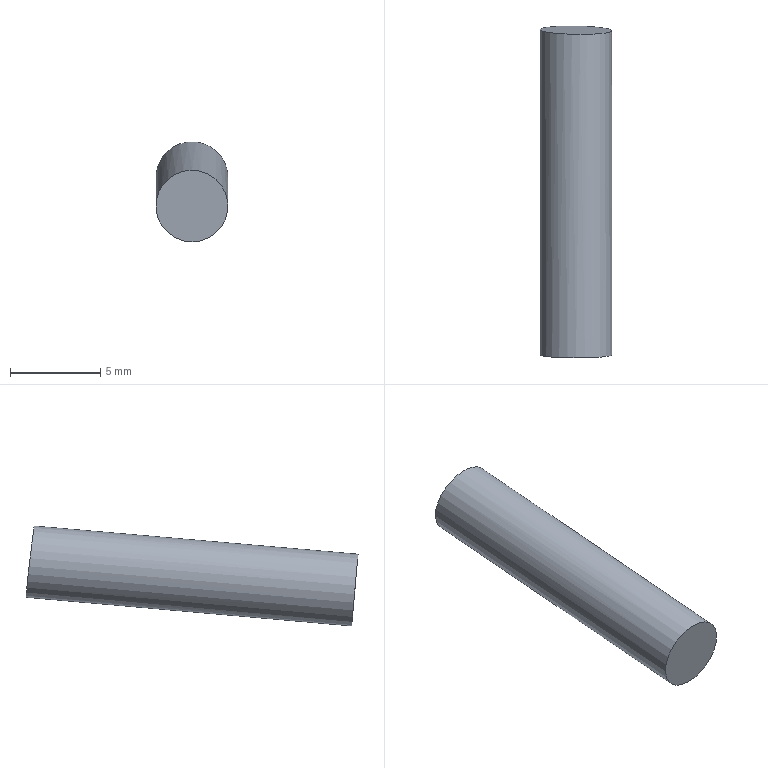Part | NX | features solid 2 | 1 solid | 3 faces | box 4 x 18.427 x 5.556 mm | volume 227.287 mm3 | plane 2 | cylinder 1 | commonest cylinder face diameters 4 x1
STEP:
#1=CARTESIAN_POINT('',(208.737,39.911,-47.538));
#2=VERTEX_POINT('',#1);
#3=CARTESIAN_POINT('',(208.737,39.736,-45.546));
#4=DIRECTION('',(0.,-0.9962,-0.08716));
#5=DIRECTION('',(0.,0.08716,-0.9962));
#6=AXIS2_PLACEMENT_3D('',#3,#4,#5);
#7=CIRCLE('',#6,2.);
#8=EDGE_CURVE('',#2,#2,#7,.T.);
#9=ORIENTED_EDGE('',*,*,#8,.T.);
#10=EDGE_LOOP('',(#9));
#11=FACE_BOUND('',#10,.T.);
#12=CARTESIAN_POINT('',(208.737,39.736,-45.546));
#13=DIRECTION('',(0.,-0.9962,-0.08716));
#14=DIRECTION('',(0.,-0.08716,0.9962));
#15=AXIS2_PLACEMENT_3D('',#12,#13,#14);
#16=PLANE('',#15);
#17=ADVANCED_FACE('',(#11),#16,.T.);
#18=CARTESIAN_POINT('',(209.678,57.535,-42.217));
#19=VERTEX_POINT('',#18);
#20=CARTESIAN_POINT('',(208.737,57.754,-43.969));
#21=DIRECTION('',(0.01549,0.9931,0.116));
#22=DIRECTION('',(0.4705,-0.1096,0.8755));
#23=AXIS2_PLACEMENT_3D('',#20,#21,#22);
#24=ELLIPSE('',#23,2.001,2.);
#25=EDGE_CURVE('',#19,#19,#24,.T.);
#26=ORIENTED_EDGE('',*,*,#25,.T.);
#27=EDGE_LOOP('',(#26));
#28=FACE_BOUND('',#27,.T.);
#29=CARTESIAN_POINT('',(159.246,62.921,-81.584));
#30=DIRECTION('',(0.01549,0.9931,0.116));
#31=DIRECTION('',(0.06594,-0.1168,0.991));
#32=AXIS2_PLACEMENT_3D('',#29,#30,#31);
#33=PLANE('',#32);
#34=ADVANCED_FACE('',(#28),#33,.T.);
#35=ORIENTED_EDGE('',*,*,#8,.F.);
#36=EDGE_LOOP('',(#35));
#37=FACE_BOUND('',#36,.T.);
#38=ORIENTED_EDGE('',*,*,#25,.F.);
#39=EDGE_LOOP('',(#38));
#40=FACE_BOUND('',#39,.T.);
#41=CARTESIAN_POINT('',(208.737,59.66,-43.803));
#42=DIRECTION('',(0.,-0.9962,-0.08716));
#43=DIRECTION('',(0.,-0.08716,0.9962));
#44=AXIS2_PLACEMENT_3D('',#41,#42,#43);
#45=CYLINDRICAL_SURFACE('',#44,2.);
#46=ADVANCED_FACE('',(#37,#40),#45,.T.);
#47=CLOSED_SHELL('',(#17,#34,#46));
#48=MANIFOLD_SOLID_BREP('',#47);
#49=(LENGTH_UNIT()NAMED_UNIT(*)SI_UNIT(.MILLI.,.METRE.));
#50=UNCERTAINTY_MEASURE_WITH_UNIT(LENGTH_MEASURE(0.00001),#49,'','');
#51=(NAMED_UNIT(*)PLANE_ANGLE_UNIT()SI_UNIT($,.RADIAN.));
#52=(NAMED_UNIT(*)SI_UNIT($,.STERADIAN.)SOLID_ANGLE_UNIT());
#53=(GEOMETRIC_REPRESENTATION_CONTEXT(3)GLOBAL_UNCERTAINTY_ASSIGNED_CONTEXT((#50))GLOBAL_UNIT_ASSIGNED_CONTEXT((#49,#51,#52))REPRESENTATION_CONTEXT('',''));
#54=ADVANCED_BREP_SHAPE_REPRESENTATION('',(#48),#53);